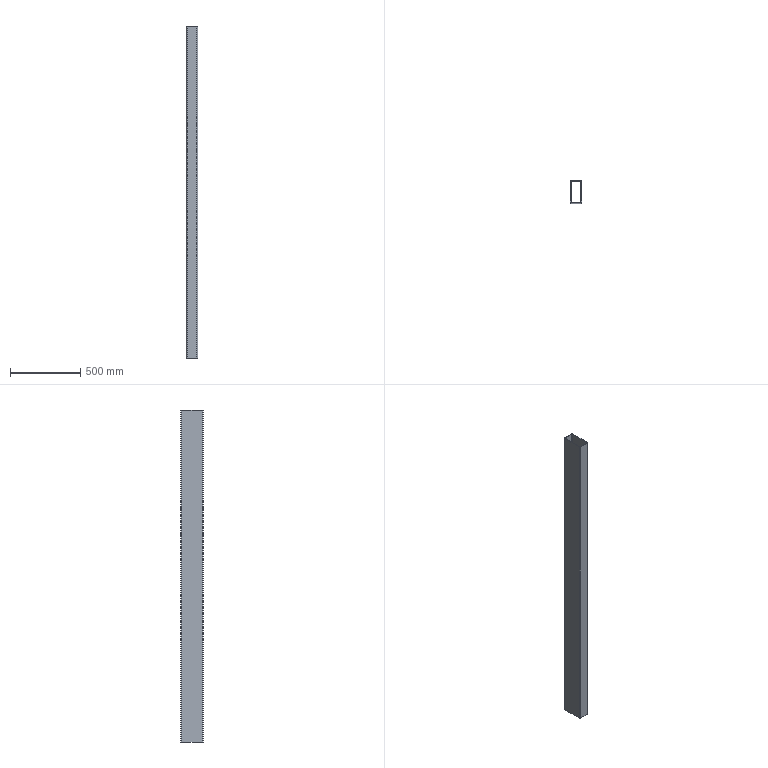Part | STEP file | 750038150 | 1 solid | 18 faces | box 80 x 160 x 2355 mm | volume 5325530 mm3 | plane 10 | cylinder 8 | commonest cylinder face diameters 4 x4 14 x4
STEP:
#1=CARTESIAN_POINT('',(-35.,73.,2355.));
#2=VERTEX_POINT('',#1);
#3=CARTESIAN_POINT('',(-35.,73.,0.));
#4=VERTEX_POINT('',#3);
#5=CARTESIAN_POINT('',(-35.,73.,2355.));
#6=DIRECTION('',(0.,0.,-1.));
#7=VECTOR('',#6,1000.);
#8=LINE('',#5,#7);
#9=EDGE_CURVE('',#2,#4,#8,.T.);
#10=ORIENTED_EDGE('',*,*,#9,.F.);
#11=CARTESIAN_POINT('',(-35.,-73.,2355.));
#12=VERTEX_POINT('',#11);
#13=CARTESIAN_POINT('',(-35.,-73.,2355.));
#14=DIRECTION('',(0.,1.,0.));
#15=VECTOR('',#14,1000.);
#16=LINE('',#13,#15);
#17=EDGE_CURVE('',#12,#2,#16,.T.);
#18=ORIENTED_EDGE('',*,*,#17,.F.);
#19=CARTESIAN_POINT('',(-35.,-73.,0.));
#20=VERTEX_POINT('',#19);
#21=CARTESIAN_POINT('',(-35.,-73.,2355.));
#22=DIRECTION('',(0.,0.,1.));
#23=VECTOR('',#22,1000.);
#24=LINE('',#21,#23);
#25=EDGE_CURVE('',#20,#12,#24,.T.);
#26=ORIENTED_EDGE('',*,*,#25,.F.);
#27=CARTESIAN_POINT('',(-35.,-73.,0.));
#28=DIRECTION('',(0.,-1.,0.));
#29=VECTOR('',#28,1000.);
#30=LINE('',#27,#29);
#31=EDGE_CURVE('',#4,#20,#30,.T.);
#32=ORIENTED_EDGE('',*,*,#31,.F.);
#33=EDGE_LOOP('',(#10,#18,#26,#32));
#34=FACE_OUTER_BOUND('',#33,.T.);
#35=CARTESIAN_POINT('',(-35.,-73.,2355.));
#36=DIRECTION('',(-1.,0.,0.));
#37=DIRECTION('',(0.,-1.,0.));
#38=AXIS2_PLACEMENT_3D('',#35,#36,#37);
#39=PLANE('',#38);
#40=ADVANCED_FACE('',(#34),#39,.F.);
#41=CARTESIAN_POINT('',(35.,73.,0.));
#42=VERTEX_POINT('',#41);
#43=CARTESIAN_POINT('',(33.,75.,0.));
#44=VERTEX_POINT('',#43);
#45=CARTESIAN_POINT('',(33.,73.,0.));
#46=DIRECTION('',(0.,0.,1.));
#47=DIRECTION('',(-1.,0.,0.));
#48=AXIS2_PLACEMENT_3D('',#45,#46,#47);
#49=CIRCLE('',#48,2.);
#50=EDGE_CURVE('',#42,#44,#49,.T.);
#51=ORIENTED_EDGE('',*,*,#50,.T.);
#52=CARTESIAN_POINT('',(-33.,75.,0.));
#53=VERTEX_POINT('',#52);
#54=CARTESIAN_POINT('',(33.,75.,0.));
#55=DIRECTION('',(-1.,0.,0.));
#56=VECTOR('',#55,1000.);
#57=LINE('',#54,#56);
#58=EDGE_CURVE('',#44,#53,#57,.T.);
#59=ORIENTED_EDGE('',*,*,#58,.T.);
#60=CARTESIAN_POINT('',(-33.,73.,0.));
#61=DIRECTION('',(0.,0.,1.));
#62=DIRECTION('',(-1.,0.,0.));
#63=AXIS2_PLACEMENT_3D('',#60,#61,#62);
#64=CIRCLE('',#63,2.);
#65=EDGE_CURVE('',#53,#4,#64,.T.);
#66=ORIENTED_EDGE('',*,*,#65,.T.);
#67=ORIENTED_EDGE('',*,*,#31,.T.);
#68=CARTESIAN_POINT('',(-33.,-75.,0.));
#69=VERTEX_POINT('',#68);
#70=CARTESIAN_POINT('',(-33.,-73.,0.));
#71=DIRECTION('',(0.,0.,1.));
#72=DIRECTION('',(-1.,0.,0.));
#73=AXIS2_PLACEMENT_3D('',#70,#71,#72);
#74=CIRCLE('',#73,2.);
#75=EDGE_CURVE('',#20,#69,#74,.T.);
#76=ORIENTED_EDGE('',*,*,#75,.T.);
#77=CARTESIAN_POINT('',(33.,-75.,0.));
#78=VERTEX_POINT('',#77);
#79=CARTESIAN_POINT('',(33.,-75.,0.));
#80=DIRECTION('',(1.,0.,0.));
#81=VECTOR('',#80,1000.);
#82=LINE('',#79,#81);
#83=EDGE_CURVE('',#69,#78,#82,.T.);
#84=ORIENTED_EDGE('',*,*,#83,.T.);
#85=CARTESIAN_POINT('',(35.,-73.,0.));
#86=VERTEX_POINT('',#85);
#87=CARTESIAN_POINT('',(33.,-73.,0.));
#88=DIRECTION('',(0.,0.,1.));
#89=DIRECTION('',(-1.,0.,0.));
#90=AXIS2_PLACEMENT_3D('',#87,#88,#89);
#91=CIRCLE('',#90,2.);
#92=EDGE_CURVE('',#78,#86,#91,.T.);
#93=ORIENTED_EDGE('',*,*,#92,.T.);
#94=CARTESIAN_POINT('',(35.,-73.,0.));
#95=DIRECTION('',(0.,1.,0.));
#96=VECTOR('',#95,1000.);
#97=LINE('',#94,#96);
#98=EDGE_CURVE('',#86,#42,#97,.T.);
#99=ORIENTED_EDGE('',*,*,#98,.T.);
#100=EDGE_LOOP('',(#51,#59,#66,#67,#76,#84,#93,#99));
#101=FACE_BOUND('',#100,.T.);
#102=CARTESIAN_POINT('',(-33.,80.,0.));
#103=VERTEX_POINT('',#102);
#104=CARTESIAN_POINT('',(33.,80.,0.));
#105=VERTEX_POINT('',#104);
#106=CARTESIAN_POINT('',(33.,80.,0.));
#107=DIRECTION('',(1.,0.,0.));
#108=VECTOR('',#107,1000.);
#109=LINE('',#106,#108);
#110=EDGE_CURVE('',#103,#105,#109,.T.);
#111=ORIENTED_EDGE('',*,*,#110,.T.);
#112=CARTESIAN_POINT('',(40.,73.,0.));
#113=VERTEX_POINT('',#112);
#114=CARTESIAN_POINT('',(33.,73.,0.));
#115=DIRECTION('',(0.,0.,-1.));
#116=DIRECTION('',(-1.,0.,0.));
#117=AXIS2_PLACEMENT_3D('',#114,#115,#116);
#118=CIRCLE('',#117,7.);
#119=EDGE_CURVE('',#105,#113,#118,.T.);
#120=ORIENTED_EDGE('',*,*,#119,.T.);
#121=CARTESIAN_POINT('',(40.,-73.,0.));
#122=VERTEX_POINT('',#121);
#123=CARTESIAN_POINT('',(40.,-73.,0.));
#124=DIRECTION('',(0.,-1.,0.));
#125=VECTOR('',#124,1000.);
#126=LINE('',#123,#125);
#127=EDGE_CURVE('',#113,#122,#126,.T.);
#128=ORIENTED_EDGE('',*,*,#127,.T.);
#129=CARTESIAN_POINT('',(33.,-80.,0.));
#130=VERTEX_POINT('',#129);
#131=CARTESIAN_POINT('',(33.,-73.,0.));
#132=DIRECTION('',(0.,0.,-1.));
#133=DIRECTION('',(-1.,0.,0.));
#134=AXIS2_PLACEMENT_3D('',#131,#132,#133);
#135=CIRCLE('',#134,7.);
#136=EDGE_CURVE('',#122,#130,#135,.T.);
#137=ORIENTED_EDGE('',*,*,#136,.T.);
#138=CARTESIAN_POINT('',(-33.,-80.,0.));
#139=VERTEX_POINT('',#138);
#140=CARTESIAN_POINT('',(33.,-80.,0.));
#141=DIRECTION('',(-1.,0.,0.));
#142=VECTOR('',#141,1000.);
#143=LINE('',#140,#142);
#144=EDGE_CURVE('',#130,#139,#143,.T.);
#145=ORIENTED_EDGE('',*,*,#144,.T.);
#146=CARTESIAN_POINT('',(-40.,-73.,0.));
#147=VERTEX_POINT('',#146);
#148=CARTESIAN_POINT('',(-33.,-73.,0.));
#149=DIRECTION('',(0.,0.,-1.));
#150=DIRECTION('',(-1.,0.,0.));
#151=AXIS2_PLACEMENT_3D('',#148,#149,#150);
#152=CIRCLE('',#151,7.);
#153=EDGE_CURVE('',#139,#147,#152,.T.);
#154=ORIENTED_EDGE('',*,*,#153,.T.);
#155=CARTESIAN_POINT('',(-40.,73.,0.));
#156=VERTEX_POINT('',#155);
#157=CARTESIAN_POINT('',(-40.,-73.,0.));
#158=DIRECTION('',(0.,1.,0.));
#159=VECTOR('',#158,1000.);
#160=LINE('',#157,#159);
#161=EDGE_CURVE('',#147,#156,#160,.T.);
#162=ORIENTED_EDGE('',*,*,#161,.T.);
#163=CARTESIAN_POINT('',(-33.,73.,0.));
#164=DIRECTION('',(0.,0.,-1.));
#165=DIRECTION('',(-1.,0.,0.));
#166=AXIS2_PLACEMENT_3D('',#163,#164,#165);
#167=CIRCLE('',#166,7.);
#168=EDGE_CURVE('',#156,#103,#167,.T.);
#169=ORIENTED_EDGE('',*,*,#168,.T.);
#170=EDGE_LOOP('',(#111,#120,#128,#137,#145,#154,#162,#169));
#171=FACE_OUTER_BOUND('',#170,.T.);
#172=CARTESIAN_POINT('',(33.,-73.,0.));
#173=DIRECTION('',(0.,0.,-1.));
#174=DIRECTION('',(-1.,0.,0.));
#175=AXIS2_PLACEMENT_3D('',#172,#173,#174);
#176=PLANE('',#175);
#177=ADVANCED_FACE('',(#101,#171),#176,.T.);
#178=CARTESIAN_POINT('',(-33.,75.,2355.));
#179=VERTEX_POINT('',#178);
#180=CARTESIAN_POINT('',(-33.,75.,2355.));
#181=DIRECTION('',(0.,0.,-1.));
#182=VECTOR('',#181,1000.);
#183=LINE('',#180,#182);
#184=EDGE_CURVE('',#179,#53,#183,.T.);
#185=ORIENTED_EDGE('',*,*,#184,.F.);
#186=CARTESIAN_POINT('',(-33.,73.,2355.));
#187=DIRECTION('',(0.,0.,-1.));
#188=DIRECTION('',(-1.,0.,0.));
#189=AXIS2_PLACEMENT_3D('',#186,#187,#188);
#190=CIRCLE('',#189,2.);
#191=EDGE_CURVE('',#2,#179,#190,.T.);
#192=ORIENTED_EDGE('',*,*,#191,.F.);
#193=ORIENTED_EDGE('',*,*,#9,.T.);
#194=ORIENTED_EDGE('',*,*,#65,.F.);
#195=EDGE_LOOP('',(#185,#192,#193,#194));
#196=FACE_OUTER_BOUND('',#195,.T.);
#197=CARTESIAN_POINT('',(-33.,73.,2355.));
#198=DIRECTION('',(0.,0.,-1.));
#199=DIRECTION('',(-1.,0.,0.));
#200=AXIS2_PLACEMENT_3D('',#197,#198,#199);
#201=CYLINDRICAL_SURFACE('',#200,2.);
#202=ADVANCED_FACE('',(#196),#201,.F.);
#203=CARTESIAN_POINT('',(33.,75.,2355.));
#204=VERTEX_POINT('',#203);
#205=CARTESIAN_POINT('',(33.,75.,2355.));
#206=DIRECTION('',(-1.,0.,0.));
#207=VECTOR('',#206,1000.);
#208=LINE('',#205,#207);
#209=EDGE_CURVE('',#204,#179,#208,.T.);
#210=ORIENTED_EDGE('',*,*,#209,.F.);
#211=CARTESIAN_POINT('',(35.,73.,2355.));
#212=VERTEX_POINT('',#211);
#213=CARTESIAN_POINT('',(33.,73.,2355.));
#214=DIRECTION('',(0.,0.,1.));
#215=DIRECTION('',(-1.,0.,0.));
#216=AXIS2_PLACEMENT_3D('',#213,#214,#215);
#217=CIRCLE('',#216,2.);
#218=EDGE_CURVE('',#212,#204,#217,.T.);
#219=ORIENTED_EDGE('',*,*,#218,.F.);
#220=CARTESIAN_POINT('',(35.,-73.,2355.));
#221=VERTEX_POINT('',#220);
#222=CARTESIAN_POINT('',(35.,-73.,2355.));
#223=DIRECTION('',(0.,1.,0.));
#224=VECTOR('',#223,1000.);
#225=LINE('',#222,#224);
#226=EDGE_CURVE('',#221,#212,#225,.T.);
#227=ORIENTED_EDGE('',*,*,#226,.F.);
#228=CARTESIAN_POINT('',(33.,-75.,2355.));
#229=VERTEX_POINT('',#228);
#230=CARTESIAN_POINT('',(33.,-73.,2355.));
#231=DIRECTION('',(0.,0.,1.));
#232=DIRECTION('',(-1.,0.,0.));
#233=AXIS2_PLACEMENT_3D('',#230,#231,#232);
#234=CIRCLE('',#233,2.);
#235=EDGE_CURVE('',#229,#221,#234,.T.);
#236=ORIENTED_EDGE('',*,*,#235,.F.);
#237=CARTESIAN_POINT('',(-33.,-75.,2355.));
#238=VERTEX_POINT('',#237);
#239=CARTESIAN_POINT('',(33.,-75.,2355.));
#240=DIRECTION('',(1.,0.,0.));
#241=VECTOR('',#240,1000.);
#242=LINE('',#239,#241);
#243=EDGE_CURVE('',#238,#229,#242,.T.);
#244=ORIENTED_EDGE('',*,*,#243,.F.);
#245=CARTESIAN_POINT('',(-33.,-73.,2355.));
#246=DIRECTION('',(0.,0.,1.));
#247=DIRECTION('',(-1.,0.,0.));
#248=AXIS2_PLACEMENT_3D('',#245,#246,#247);
#249=CIRCLE('',#248,2.);
#250=EDGE_CURVE('',#12,#238,#249,.T.);
#251=ORIENTED_EDGE('',*,*,#250,.F.);
#252=ORIENTED_EDGE('',*,*,#17,.T.);
#253=ORIENTED_EDGE('',*,*,#191,.T.);
#254=EDGE_LOOP('',(#210,#219,#227,#236,#244,#251,#252,#253));
#255=FACE_BOUND('',#254,.T.);
#256=CARTESIAN_POINT('',(33.,80.,2355.));
#257=VERTEX_POINT('',#256);
#258=CARTESIAN_POINT('',(40.,73.,2355.));
#259=VERTEX_POINT('',#258);
#260=CARTESIAN_POINT('',(33.,73.,2355.));
#261=DIRECTION('',(0.,0.,-1.));
#262=DIRECTION('',(-1.,0.,0.));
#263=AXIS2_PLACEMENT_3D('',#260,#261,#262);
#264=CIRCLE('',#263,7.);
#265=EDGE_CURVE('',#257,#259,#264,.T.);
#266=ORIENTED_EDGE('',*,*,#265,.F.);
#267=CARTESIAN_POINT('',(-33.,80.,2355.));
#268=VERTEX_POINT('',#267);
#269=CARTESIAN_POINT('',(33.,80.,2355.));
#270=DIRECTION('',(1.,0.,0.));
#271=VECTOR('',#270,1000.);
#272=LINE('',#269,#271);
#273=EDGE_CURVE('',#268,#257,#272,.T.);
#274=ORIENTED_EDGE('',*,*,#273,.F.);
#275=CARTESIAN_POINT('',(-40.,73.,2355.));
#276=VERTEX_POINT('',#275);
#277=CARTESIAN_POINT('',(-33.,73.,2355.));
#278=DIRECTION('',(0.,0.,-1.));
#279=DIRECTION('',(-1.,0.,0.));
#280=AXIS2_PLACEMENT_3D('',#277,#278,#279);
#281=CIRCLE('',#280,7.);
#282=EDGE_CURVE('',#276,#268,#281,.T.);
#283=ORIENTED_EDGE('',*,*,#282,.F.);
#284=CARTESIAN_POINT('',(-40.,-73.,2355.));
#285=VERTEX_POINT('',#284);
#286=CARTESIAN_POINT('',(-40.,-73.,2355.));
#287=DIRECTION('',(0.,1.,0.));
#288=VECTOR('',#287,1000.);
#289=LINE('',#286,#288);
#290=EDGE_CURVE('',#285,#276,#289,.T.);
#291=ORIENTED_EDGE('',*,*,#290,.F.);
#292=CARTESIAN_POINT('',(-33.,-80.,2355.));
#293=VERTEX_POINT('',#292);
#294=CARTESIAN_POINT('',(-33.,-73.,2355.));
#295=DIRECTION('',(0.,0.,-1.));
#296=DIRECTION('',(-1.,0.,0.));
#297=AXIS2_PLACEMENT_3D('',#294,#295,#296);
#298=CIRCLE('',#297,7.);
#299=EDGE_CURVE('',#293,#285,#298,.T.);
#300=ORIENTED_EDGE('',*,*,#299,.F.);
#301=CARTESIAN_POINT('',(33.,-80.,2355.));
#302=VERTEX_POINT('',#301);
#303=CARTESIAN_POINT('',(33.,-80.,2355.));
#304=DIRECTION('',(-1.,0.,0.));
#305=VECTOR('',#304,1000.);
#306=LINE('',#303,#305);
#307=EDGE_CURVE('',#302,#293,#306,.T.);
#308=ORIENTED_EDGE('',*,*,#307,.F.);
#309=CARTESIAN_POINT('',(40.,-73.,2355.));
#310=VERTEX_POINT('',#309);
#311=CARTESIAN_POINT('',(33.,-73.,2355.));
#312=DIRECTION('',(0.,0.,-1.));
#313=DIRECTION('',(-1.,0.,0.));
#314=AXIS2_PLACEMENT_3D('',#311,#312,#313);
#315=CIRCLE('',#314,7.);
#316=EDGE_CURVE('',#310,#302,#315,.T.);
#317=ORIENTED_EDGE('',*,*,#316,.F.);
#318=CARTESIAN_POINT('',(40.,-73.,2355.));
#319=DIRECTION('',(0.,-1.,0.));
#320=VECTOR('',#319,1000.);
#321=LINE('',#318,#320);
#322=EDGE_CURVE('',#259,#310,#321,.T.);
#323=ORIENTED_EDGE('',*,*,#322,.F.);
#324=EDGE_LOOP('',(#266,#274,#283,#291,#300,#308,#317,#323));
#325=FACE_OUTER_BOUND('',#324,.T.);
#326=CARTESIAN_POINT('',(33.,-73.,2355.));
#327=DIRECTION('',(0.,0.,-1.));
#328=DIRECTION('',(-1.,0.,0.));
#329=AXIS2_PLACEMENT_3D('',#326,#327,#328);
#330=PLANE('',#329);
#331=ADVANCED_FACE('',(#255,#325),#330,.F.);
#332=ORIENTED_EDGE('',*,*,#25,.T.);
#333=ORIENTED_EDGE('',*,*,#250,.T.);
#334=CARTESIAN_POINT('',(-33.,-75.,2355.));
#335=DIRECTION('',(0.,0.,1.));
#336=VECTOR('',#335,1000.);
#337=LINE('',#334,#336);
#338=EDGE_CURVE('',#69,#238,#337,.T.);
#339=ORIENTED_EDGE('',*,*,#338,.F.);
#340=ORIENTED_EDGE('',*,*,#75,.F.);
#341=EDGE_LOOP('',(#332,#333,#339,#340));
#342=FACE_OUTER_BOUND('',#341,.T.);
#343=CARTESIAN_POINT('',(-33.,-73.,2355.));
#344=DIRECTION('',(0.,0.,-1.));
#345=DIRECTION('',(-1.,0.,0.));
#346=AXIS2_PLACEMENT_3D('',#343,#344,#345);
#347=CYLINDRICAL_SURFACE('',#346,2.);
#348=ADVANCED_FACE('',(#342),#347,.F.);
#349=CARTESIAN_POINT('',(33.,75.,2355.));
#350=DIRECTION('',(0.,0.,-1.));
#351=VECTOR('',#350,1000.);
#352=LINE('',#349,#351);
#353=EDGE_CURVE('',#204,#44,#352,.T.);
#354=ORIENTED_EDGE('',*,*,#353,.F.);
#355=ORIENTED_EDGE('',*,*,#209,.T.);
#356=ORIENTED_EDGE('',*,*,#184,.T.);
#357=ORIENTED_EDGE('',*,*,#58,.F.);
#358=EDGE_LOOP('',(#354,#355,#356,#357));
#359=FACE_OUTER_BOUND('',#358,.T.);
#360=CARTESIAN_POINT('',(-33.,75.,2355.));
#361=DIRECTION('',(0.,1.,0.));
#362=DIRECTION('',(0.,0.,1.));
#363=AXIS2_PLACEMENT_3D('',#360,#361,#362);
#364=PLANE('',#363);
#365=ADVANCED_FACE('',(#359),#364,.F.);
#366=CARTESIAN_POINT('',(35.,73.,2355.));
#367=DIRECTION('',(0.,0.,-1.));
#368=VECTOR('',#367,1000.);
#369=LINE('',#366,#368);
#370=EDGE_CURVE('',#212,#42,#369,.T.);
#371=ORIENTED_EDGE('',*,*,#370,.F.);
#372=ORIENTED_EDGE('',*,*,#218,.T.);
#373=ORIENTED_EDGE('',*,*,#353,.T.);
#374=ORIENTED_EDGE('',*,*,#50,.F.);
#375=EDGE_LOOP('',(#371,#372,#373,#374));
#376=FACE_OUTER_BOUND('',#375,.T.);
#377=CARTESIAN_POINT('',(33.,73.,2355.));
#378=DIRECTION('',(0.,0.,-1.));
#379=DIRECTION('',(-1.,0.,0.));
#380=AXIS2_PLACEMENT_3D('',#377,#378,#379);
#381=CYLINDRICAL_SURFACE('',#380,2.);
#382=ADVANCED_FACE('',(#376),#381,.F.);
#383=CARTESIAN_POINT('',(35.,-73.,2355.));
#384=DIRECTION('',(0.,0.,-1.));
#385=VECTOR('',#384,1000.);
#386=LINE('',#383,#385);
#387=EDGE_CURVE('',#221,#86,#386,.T.);
#388=ORIENTED_EDGE('',*,*,#387,.F.);
#389=ORIENTED_EDGE('',*,*,#226,.T.);
#390=ORIENTED_EDGE('',*,*,#370,.T.);
#391=ORIENTED_EDGE('',*,*,#98,.F.);
#392=EDGE_LOOP('',(#388,#389,#390,#391));
#393=FACE_OUTER_BOUND('',#392,.T.);
#394=CARTESIAN_POINT('',(35.,73.,2355.));
#395=DIRECTION('',(1.,0.,0.));
#396=DIRECTION('',(0.,1.,0.));
#397=AXIS2_PLACEMENT_3D('',#394,#395,#396);
#398=PLANE('',#397);
#399=ADVANCED_FACE('',(#393),#398,.F.);
#400=CARTESIAN_POINT('',(33.,-75.,2355.));
#401=DIRECTION('',(0.,0.,-1.));
#402=VECTOR('',#401,1000.);
#403=LINE('',#400,#402);
#404=EDGE_CURVE('',#229,#78,#403,.T.);
#405=ORIENTED_EDGE('',*,*,#404,.F.);
#406=ORIENTED_EDGE('',*,*,#235,.T.);
#407=ORIENTED_EDGE('',*,*,#387,.T.);
#408=ORIENTED_EDGE('',*,*,#92,.F.);
#409=EDGE_LOOP('',(#405,#406,#407,#408));
#410=FACE_OUTER_BOUND('',#409,.T.);
#411=CARTESIAN_POINT('',(33.,-73.,2355.));
#412=DIRECTION('',(0.,0.,-1.));
#413=DIRECTION('',(-1.,0.,0.));
#414=AXIS2_PLACEMENT_3D('',#411,#412,#413);
#415=CYLINDRICAL_SURFACE('',#414,2.);
#416=ADVANCED_FACE('',(#410),#415,.F.);
#417=ORIENTED_EDGE('',*,*,#338,.T.);
#418=ORIENTED_EDGE('',*,*,#243,.T.);
#419=ORIENTED_EDGE('',*,*,#404,.T.);
#420=ORIENTED_EDGE('',*,*,#83,.F.);
#421=EDGE_LOOP('',(#417,#418,#419,#420));
#422=FACE_OUTER_BOUND('',#421,.T.);
#423=CARTESIAN_POINT('',(33.,-75.,2355.));
#424=DIRECTION('',(0.,-1.,0.));
#425=DIRECTION('',(0.,0.,-1.));
#426=AXIS2_PLACEMENT_3D('',#423,#424,#425);
#427=PLANE('',#426);
#428=ADVANCED_FACE('',(#422),#427,.F.);
#429=ORIENTED_EDGE('',*,*,#265,.T.);
#430=CARTESIAN_POINT('',(40.,73.,2355.));
#431=DIRECTION('',(0.,0.,-1.));
#432=VECTOR('',#431,1000.);
#433=LINE('',#430,#432);
#434=EDGE_CURVE('',#259,#113,#433,.T.);
#435=ORIENTED_EDGE('',*,*,#434,.T.);
#436=ORIENTED_EDGE('',*,*,#119,.F.);
#437=CARTESIAN_POINT('',(33.,80.,2355.));
#438=DIRECTION('',(0.,0.,1.));
#439=VECTOR('',#438,1000.);
#440=LINE('',#437,#439);
#441=EDGE_CURVE('',#105,#257,#440,.T.);
#442=ORIENTED_EDGE('',*,*,#441,.T.);
#443=EDGE_LOOP('',(#429,#435,#436,#442));
#444=FACE_OUTER_BOUND('',#443,.T.);
#445=CARTESIAN_POINT('',(33.,73.,2355.));
#446=DIRECTION('',(0.,0.,-1.));
#447=DIRECTION('',(-1.,0.,0.));
#448=AXIS2_PLACEMENT_3D('',#445,#446,#447);
#449=CYLINDRICAL_SURFACE('',#448,7.);
#450=ADVANCED_FACE('',(#444),#449,.T.);
#451=ORIENTED_EDGE('',*,*,#273,.T.);
#452=ORIENTED_EDGE('',*,*,#441,.F.);
#453=ORIENTED_EDGE('',*,*,#110,.F.);
#454=CARTESIAN_POINT('',(-33.,80.,2355.));
#455=DIRECTION('',(0.,0.,1.));
#456=VECTOR('',#455,1000.);
#457=LINE('',#454,#456);
#458=EDGE_CURVE('',#103,#268,#457,.T.);
#459=ORIENTED_EDGE('',*,*,#458,.T.);
#460=EDGE_LOOP('',(#451,#452,#453,#459));
#461=FACE_OUTER_BOUND('',#460,.T.);
#462=CARTESIAN_POINT('',(-33.,80.,2355.));
#463=DIRECTION('',(0.,1.,0.));
#464=DIRECTION('',(0.,0.,1.));
#465=AXIS2_PLACEMENT_3D('',#462,#463,#464);
#466=PLANE('',#465);
#467=ADVANCED_FACE('',(#461),#466,.T.);
#468=ORIENTED_EDGE('',*,*,#282,.T.);
#469=ORIENTED_EDGE('',*,*,#458,.F.);
#470=ORIENTED_EDGE('',*,*,#168,.F.);
#471=CARTESIAN_POINT('',(-40.,73.,2355.));
#472=DIRECTION('',(0.,0.,1.));
#473=VECTOR('',#472,1000.);
#474=LINE('',#471,#473);
#475=EDGE_CURVE('',#156,#276,#474,.T.);
#476=ORIENTED_EDGE('',*,*,#475,.T.);
#477=EDGE_LOOP('',(#468,#469,#470,#476));
#478=FACE_OUTER_BOUND('',#477,.T.);
#479=CARTESIAN_POINT('',(-33.,73.,2355.));
#480=DIRECTION('',(0.,0.,-1.));
#481=DIRECTION('',(-1.,0.,0.));
#482=AXIS2_PLACEMENT_3D('',#479,#480,#481);
#483=CYLINDRICAL_SURFACE('',#482,7.);
#484=ADVANCED_FACE('',(#478),#483,.T.);
#485=ORIENTED_EDGE('',*,*,#290,.T.);
#486=ORIENTED_EDGE('',*,*,#475,.F.);
#487=ORIENTED_EDGE('',*,*,#161,.F.);
#488=CARTESIAN_POINT('',(-40.,-73.,2355.));
#489=DIRECTION('',(0.,0.,1.));
#490=VECTOR('',#489,1000.);
#491=LINE('',#488,#490);
#492=EDGE_CURVE('',#147,#285,#491,.T.);
#493=ORIENTED_EDGE('',*,*,#492,.T.);
#494=EDGE_LOOP('',(#485,#486,#487,#493));
#495=FACE_OUTER_BOUND('',#494,.T.);
#496=CARTESIAN_POINT('',(-40.,-73.,2355.));
#497=DIRECTION('',(-1.,0.,0.));
#498=DIRECTION('',(0.,0.,1.));
#499=AXIS2_PLACEMENT_3D('',#496,#497,#498);
#500=PLANE('',#499);
#501=ADVANCED_FACE('',(#495),#500,.T.);
#502=ORIENTED_EDGE('',*,*,#299,.T.);
#503=ORIENTED_EDGE('',*,*,#492,.F.);
#504=ORIENTED_EDGE('',*,*,#153,.F.);
#505=CARTESIAN_POINT('',(-33.,-80.,2355.));
#506=DIRECTION('',(0.,0.,1.));
#507=VECTOR('',#506,1000.);
#508=LINE('',#505,#507);
#509=EDGE_CURVE('',#139,#293,#508,.T.);
#510=ORIENTED_EDGE('',*,*,#509,.T.);
#511=EDGE_LOOP('',(#502,#503,#504,#510));
#512=FACE_OUTER_BOUND('',#511,.T.);
#513=CARTESIAN_POINT('',(-33.,-73.,2355.));
#514=DIRECTION('',(0.,0.,-1.));
#515=DIRECTION('',(-1.,0.,0.));
#516=AXIS2_PLACEMENT_3D('',#513,#514,#515);
#517=CYLINDRICAL_SURFACE('',#516,7.);
#518=ADVANCED_FACE('',(#512),#517,.T.);
#519=ORIENTED_EDGE('',*,*,#307,.T.);
#520=ORIENTED_EDGE('',*,*,#509,.F.);
#521=ORIENTED_EDGE('',*,*,#144,.F.);
#522=CARTESIAN_POINT('',(33.,-80.,2355.));
#523=DIRECTION('',(0.,0.,1.));
#524=VECTOR('',#523,1000.);
#525=LINE('',#522,#524);
#526=EDGE_CURVE('',#130,#302,#525,.T.);
#527=ORIENTED_EDGE('',*,*,#526,.T.);
#528=EDGE_LOOP('',(#519,#520,#521,#527));
#529=FACE_OUTER_BOUND('',#528,.T.);
#530=CARTESIAN_POINT('',(33.,-80.,2355.));
#531=DIRECTION('',(0.,-1.,0.));
#532=DIRECTION('',(0.,0.,-1.));
#533=AXIS2_PLACEMENT_3D('',#530,#531,#532);
#534=PLANE('',#533);
#535=ADVANCED_FACE('',(#529),#534,.T.);
#536=ORIENTED_EDGE('',*,*,#316,.T.);
#537=ORIENTED_EDGE('',*,*,#526,.F.);
#538=ORIENTED_EDGE('',*,*,#136,.F.);
#539=CARTESIAN_POINT('',(40.,-73.,2355.));
#540=DIRECTION('',(0.,0.,1.));
#541=VECTOR('',#540,1000.);
#542=LINE('',#539,#541);
#543=EDGE_CURVE('',#122,#310,#542,.T.);
#544=ORIENTED_EDGE('',*,*,#543,.T.);
#545=EDGE_LOOP('',(#536,#537,#538,#544));
#546=FACE_OUTER_BOUND('',#545,.T.);
#547=CARTESIAN_POINT('',(33.,-73.,2355.));
#548=DIRECTION('',(0.,0.,-1.));
#549=DIRECTION('',(-1.,0.,0.));
#550=AXIS2_PLACEMENT_3D('',#547,#548,#549);
#551=CYLINDRICAL_SURFACE('',#550,7.);
#552=ADVANCED_FACE('',(#546),#551,.T.);
#553=ORIENTED_EDGE('',*,*,#322,.T.);
#554=ORIENTED_EDGE('',*,*,#543,.F.);
#555=ORIENTED_EDGE('',*,*,#127,.F.);
#556=ORIENTED_EDGE('',*,*,#434,.F.);
#557=EDGE_LOOP('',(#553,#554,#555,#556));
#558=FACE_OUTER_BOUND('',#557,.T.);
#559=CARTESIAN_POINT('',(40.,73.,2355.));
#560=DIRECTION('',(1.,0.,0.));
#561=DIRECTION('',(0.,1.,0.));
#562=AXIS2_PLACEMENT_3D('',#559,#560,#561);
#563=PLANE('',#562);
#564=ADVANCED_FACE('',(#558),#563,.T.);
#565=CLOSED_SHELL('',(#40,#177,#202,#331,#348,#365,#382,#399,#416,#428,#450,#467,#484,#501,#518,#535,#552,#564));
#566=MANIFOLD_SOLID_BREP('',#565);
#567=CARTESIAN_POINT('',(0.,0.,0.));
#568=DIRECTION('',(0.,0.,1.));
#569=DIRECTION('',(1.,0.,0.));
#570=AXIS2_PLACEMENT_3D('',#567,#568,#569);
#571=(LENGTH_UNIT()NAMED_UNIT(*)SI_UNIT(.MILLI.,.METRE.));
#572=UNCERTAINTY_MEASURE_WITH_UNIT(LENGTH_MEASURE(0.00001),#571,'','');
#573=(NAMED_UNIT(*)PLANE_ANGLE_UNIT()SI_UNIT($,.RADIAN.));
#574=(NAMED_UNIT(*)SI_UNIT($,.STERADIAN.)SOLID_ANGLE_UNIT());
#575=(GEOMETRIC_REPRESENTATION_CONTEXT(3)GLOBAL_UNCERTAINTY_ASSIGNED_CONTEXT((#572))GLOBAL_UNIT_ASSIGNED_CONTEXT((#571,#573,#574))REPRESENTATION_CONTEXT('',''));
#576=ADVANCED_BREP_SHAPE_REPRESENTATION('',(#566,#570),#575);